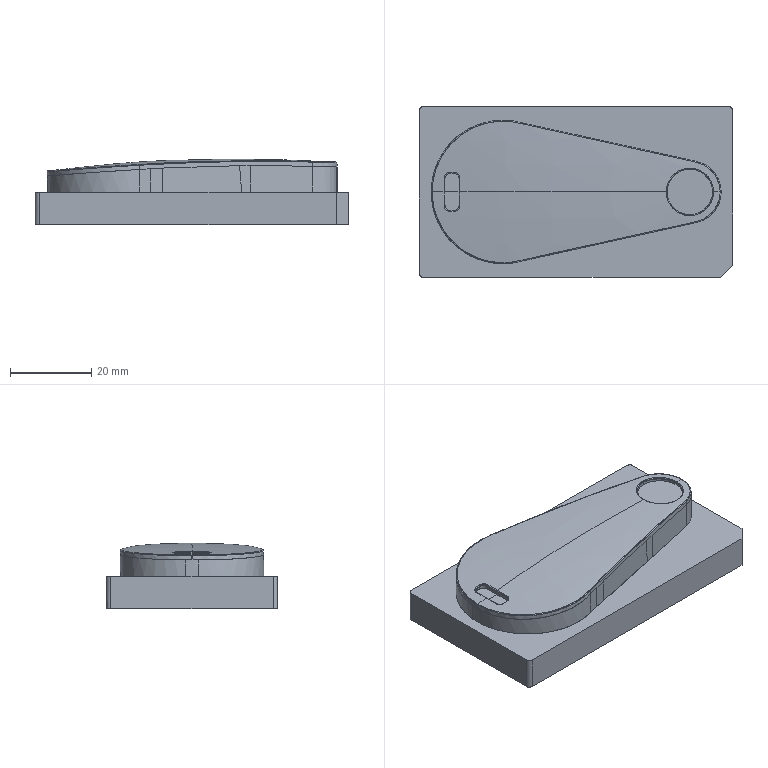NC program | PowerMill | posted with a generic post | part box 77 x 42 x 16.114 mm
Lines 1 to 941 of 134652:
%
O0001
N104 ( POWERMILL CB  : 2026004.0)
N105 ( POST VER      : 2026.0.0.5161)
N106 ( OPTION FILE   : FANUC)
N107 ( OUTPUT WORKPLANE : WORLD)
N108 (  )
N109 ( TOOL LIST )
N110 (---------------------------------------)
N111 ( NO. | ID        | DIA.| TIP RAD|LENGTH)
N112 (---------------------------------------)
N113 (    1|D10C_1_1   |10.0 |  0.0   |71.48 )
N114 (    2|D4C_2_1    | 4.0 |  0.0   |63.16 )
N115 (   28|D2C_1_1    | 2.0 |  0.0   |58.12 )
N116 (    3|D10_1_1    |10.0 |  0.0   | 71.2 )
N117 (    7|R2_2_1     | 4.0 |  2.0   | 60.4 )
N118 (   12|D2_1_1     | 2.0 |  0.0   |58.28 )
N119 (    6|R0.5_2_1   | 1.0 |  0.5   | 57.6 )
N120 (   13|TEXT_D4_1_1| 4.0 |  0.3   |63.36 )
N121 (---------------------------------------)
N122 (  )
N123 ( NUMBER OF TOOLPATHS: 15.0 )
N124 ( ESTIMATED PROGRAM DURATION: 0 HOURS 30 MIN 20 SEC)
N125 (  )
N126 G00 G21 G80 G40 G17
N127 G90
N128 G54
N129 G53 Z0.0
N130 (---------------)
N131 ( START TOOLPATH : 粗公开粗01-扫面平行-D10C )
N132 (---------------)
N133 ( TOOL NO.    :1 )
N134 ( TOOL TYPE   : ENDMILL)
N135 ( TOOL ID     : D10C_1_1)
N136 ( TOOL DIA    : 10.0 LENGTH 71.48)
N137 T1
N138 M6
N139 S8000 M03
N140 G00 G90 X0.0 Y0.0
N141 G43 Z10.6 H1
N142
N143 G05 P10000 R4
N144 X46.15 Y23.65
N145 Z1.4015
N146 G01 Z0.2015 F6000.0
N147 X41.15 F10000.0
N148 X-41.15
N149 Y17.7375
N150 X41.15
N151 Y11.825
N152 X-41.15
N153 Y5.9125
N154 X41.15
N155 Y0.0
N156 X-41.15
N157 Y-5.9125
N158 X41.15
N159 Y-11.825
N160 X-41.15
N161 Y-17.7375
N162 X41.15
N163 Y-23.65
N164 X-41.15
N165 X-46.15
N166 Z-0.197
N167 X-41.15
N168 X41.15
N169 Y-17.7375
N170 X-41.15
N171 Y-11.825
N172 X41.15
N173 Y-5.9125
N174 X-41.15
N175 Y0.0
N176 X41.15
N177 Y5.9125
N178 X-41.15
N179 Y11.825
N180 X41.15
N181 Y17.7375
N182 X-41.15
N183 Y23.65
N184 X41.15
N185 X46.15
N186 G00 Z10.6
N187 G05 P0
N188 (---------------)
N189 ( END TOOLPATH : 粗公开粗01-扫面平行-D10C )
N190 (---------------)
N191 ( START TOOLPATH : 粗公开粗01-外形偏置-D10C )
N192 (---------------)
N193 G00 X0.0415 Y-0.002 Z9.8037
N194 G05 P10000 R4
N195 X15.1122 Y-30.557
N196 Z0.5573
N197 G01 Z-0.6427 F6000.0
N198 Y-30.0295 F10000.0
N199 G03 X10.3647 Y-25.282 I-4.7475 J0.0
N200 G01 X-42.229
N201 G02 X-43.229 Y-24.282 I0.0 J1.0
N202 G01 Y-8.9867
N203 X-38.3097
N204 X-32.4189
N205 X-27.9189
N206 X-32.4189
N207 Y-12.472
N208 G03 X-30.5081 Y-14.47 I2.0 J0.0
N209 G01 X-22.4604 Y-14.8291
N210 G03 X-20.6866 Y-12.1962 I0.0829 J1.8581
N211 G01 X-21.7475 Y-9.8614
N212 G02 X-23.7344 Y-0.5015 I21.0967 J9.3693
N213 G01 X-23.7348 Y0.4347
N214 G02 X-22.8956 Y6.4023 I21.5767 J0.0088
N215 G01 X-22.6364 Y7.2526
N216 X-26.9406 Y8.5652
N217 X-22.6364 Y7.2526
N218 X-22.5842 Y7.4234
N219 G02 X-21.5821 Y10.0985 I28.7047 J-9.2284
N220 G01 X-20.6681 Y12.2256
N221 G03 X-22.4648 Y14.8251 I-1.7135 J0.7363
N222 G01 X-30.5081 Y14.466
N223 G03 X-32.4189 Y12.468 I0.0892 J-1.998
N224 G01 Y-8.9867
N225 X-38.3097
N226 Y19.8018
N227 G02 X-37.7528 Y20.3587 I0.5569 J0.0
N228 G01 X-2.203 Y20.3592
N229 G02 X-2.1341 Y19.97 I0.0 J-0.2007
N230 G01 X-4.361 Y19.1563
N231 G03 X-11.3917 Y14.9524 I7.4992 J-20.5229
N232 G01 X-12.0246 Y14.3889
N233 G03 X-16.1388 Y8.746 I10.9665 J-12.317
N234 G01 X-16.5756 Y7.7592
N235 G03 X-17.4466 Y5.3603 I17.0855 J-7.5614
N236 G01 X-17.5851 Y4.8788
N237 G03 X-18.21 Y0.4369 I15.427 J-4.4353
N238 G01 X-18.2096 Y-0.4993
N239 G03 X-16.6888 Y-7.6401 I17.5588 J0.0072
N240 G01 X-16.4205 Y-8.2422
N241 X-16.0824 Y-8.9571
N242 X-15.7125 Y-9.656
N243 X-15.4448 Y-10.1355
N244 G03 X-11.7963 Y-14.5782 I14.1498 J7.9007
N245 G01 X-10.8792 Y-15.3585
N246 G03 X-3.5709 Y-19.4506 I14.0407 J16.5038
N247 G01 X-1.9551 Y-19.9788
N248 G02 X-2.0163 Y-20.3632 I-0.0612 J-0.1873
N249 G01 X-37.7528 Y-20.3627
N250 G02 X-38.3097 Y-19.8058 I0.0 J0.5569
N251 G01 Y-8.9867
N252 X-43.229
N253 Y24.278
N254 G02 X-42.229 Y25.278 I1.0 J0.0
N255 G01 X42.312
N256 G02 X43.312 Y24.278 I0.0 J-1.0
N257 G01 Y-0.002
N258 X38.3927
N259 Y-19.8058
N260 G02 X37.8358 Y-20.3627 I-0.5569 J0.0
N261 G01 X19.3428 Y-20.3632
N262 G02 X19.3059 Y-20.0003 I0.0 J0.1833
N263 G01 X25.8243 Y-18.6576
N264 G03 X35.9604 Y-11.8793 I-3.2646 J15.8493
N265 G01 X36.1512 Y-11.5973
N266 X36.2852 Y-11.3934
N267 X36.4135 Y-11.186
N268 X36.5859 Y-10.8987
N269 X36.7924 Y-10.5378
N270 G03 X38.0247 Y-5.4294 I-8.4899 J4.7508
N271 G01 X38.0231 Y-5.3865
N272 G03 X37.0167 Y-1.4345 I-9.6578 J-0.3552
N273 G01 X36.9442 Y-1.2889
N274 X36.7974 Y-1.0108
N275 X36.6375 Y-0.74
N276 X36.5527 Y-0.6039
N277 G02 X36.5528 Y0.6042 I0.9695 J0.604
N278 G01 X36.6374 Y0.74
N279 X36.877 Y1.1579
N280 X37.0853 Y1.5923
N281 X37.228 Y1.92
N282 G03 X37.2314 Y9.6259 I-8.8607 J3.8569
N283 G01 X37.0921 Y9.9456
N284 G03 X35.1033 Y12.9253 I-9.3798 J-4.1071
N285 G01 X33.7038 Y14.3849
N286 X33.546 Y14.5438
N287 G03 X26.2035 Y18.5373 I-10.3837 J-10.3447
N288 G01 X19.3237 Y19.9965
N289 G02 X19.3617 Y20.3592 I0.038 J0.1794
N290 G01 X37.8358 Y20.3587
N291 G02 X38.3927 Y19.8018 I0.0 J-0.5569
N292 G01 Y-0.002
N293 X43.312
N294 Y-24.282
N295 G02 X42.312 Y-25.282 I-1.0 J0.0
N296 G01 X10.3647
N297 X10.096 Y-16.8337
N298 X9.3226 Y-16.8583
N299 X7.0023 Y-16.7279
N300 X6.2289 Y-16.6328
N301 X3.9086 Y-16.2963
N302 X1.5884 Y-15.9314
N303 X0.8149 Y-15.7235
N304 X0.0415 Y-15.472
N305 X-1.0167 Y-15.0838
N306 X-1.5054 Y-14.9304
N307 X-3.8256 Y-14.0783
N308 X-4.7965 Y-13.537
N309 X-6.09 Y-12.7635
N310 X-8.4662 Y-10.8994
N311 X-9.2396 Y-10.254
N312 X-10.013 Y-9.3444
N313 X-11.3207 Y-7.3496
N314 X-11.7729 Y-6.5761
N315 X-12.3692 Y-5.0293
N316 X-12.8353 Y-3.4824
N317 X-12.9849 Y-2.709
N318 X-13.1446 Y-1.1621
N319 X-13.261 Y-0.3887
N320 X-13.2613 Y0.3847
N321 X-13.1068 Y1.4875
N322 X-12.7819 Y3.4784
N323 X-12.6318 Y4.2518
N324 X-12.3829 Y5.0253
N325 X-12.0531 Y5.7987
N326 X-11.2708 Y7.3456
N327 X-10.7865 Y8.1825
N328 X-10.013 Y9.3424
N329 X-9.2396 Y10.2581
N330 X-8.4662 Y10.9107
N331 X-6.1459 Y12.7679
N332 X-5.3725 Y13.2565
N333 X-4.5991 Y13.704
N334 X-3.8256 Y14.0474
N335 X0.0415 Y15.5415
N336 X0.8149 Y15.7355
N337 X4.6821 Y16.4562
N338 X7.7758 Y16.7747
N339 X9.3226 Y16.8711
N340 X10.096 Y16.8388
N341 X10.8695 Y16.7141
N342 X13.1898 Y16.2845
N343 X20.1506 Y14.7825
N344 X24.7911 Y13.7125
N345 X27.1114 Y13.0685
N346 X27.8849 Y12.7169
N347 X28.9862 Y11.9861
N348 X30.2051 Y10.9294
N349 X31.4204 Y9.6658
N350 X32.0706 Y8.8924
N351 X32.5169 Y8.119
N352 X32.8414 Y7.3456
N353 X33.0385 Y6.5721
N354 X33.1043 Y5.7987
N355 X33.0532 Y5.0253
N356 X32.854 Y4.2518
N357 X32.5404 Y3.4784
N358 X32.0786 Y2.705
N359 X31.3653 Y1.9316
N360 X30.9786 Y1.661
N361 X30.1787 Y1.1581
N362 X29.4317 Y0.8897
N363 X28.6583 Y0.6895
N364 X28.0947 Y0.573
N365 X28.0184 Y0.5508
N366 X27.9466 Y0.5168
N367 X27.8039 Y0.4348
N368 X27.7235 Y0.3772
N369 X27.6559 Y0.3049
N370 X27.6546 Y0.3032
N371 G03 X27.8164 Y-0.4416 I0.3972 J-0.3037
N372 G01 X27.9881 Y-0.5332
N373 X28.0482 Y-0.5603
N374 X28.1114 Y-0.5793
N375 X29.4317 Y-0.8831
N376 X30.2051 Y-1.1867
N377 X30.9786 Y-1.6615
N378 X31.37 Y-1.9356
N379 X32.0818 Y-2.709
N380 X32.5426 Y-3.4824
N381 X32.8554 Y-4.2558
N382 X33.0533 Y-5.0293
N383 X33.1042 Y-5.8027
N384 X33.0378 Y-6.5761
N385 X32.8256 Y-7.3496
N386 X32.5042 Y-8.123
N387 X32.0402 Y-8.8964
N388 X31.41 Y-9.6698
N389 X30.6871 Y-10.4433
N390 X30.2051 Y-10.917
N391 X29.4317 Y-11.6072
N392 X28.6583 Y-12.2299
N393 X27.83 Y-12.7635
N394 X27.1114 Y-13.0685
N395 X26.338 Y-13.2989
N396 X24.7911 Y-13.7128
N397 X20.1506 Y-14.7825
N398 X13.1898 Y-16.2844
N399 X11.341 Y-16.6307
N400 X10.096 Y-16.8337
N401 X10.3647 Y-25.282
N402 G00 Z3.2117
N403 G01 X15.1122 Y-30.557
N404 G00 Z0.1617
N405 G01 Z-1.0383 F6000.0
N406 Y-30.0295 F10000.0
N407 G03 X10.3647 Y-25.282 I-4.7475 J0.0
N408 G01 X-30.4481
N409 X-30.0672 Y-20.5382
N410 X-29.6209 Y-14.9804
N411 G03 X-27.5814 Y-12.3027 I0.1601 J1.9936
N412 G01 X-28.0999 Y-10.8534
N413 G02 X-28.0952 Y10.9505 I30.7936 J10.8953
N414 G01 X-27.6041 Y12.3366
N415 G03 X-30.1715 Y14.8846 I-1.8852 J0.6679
N416 G01 X-31.2015 Y14.5108
N417 G03 X-32.5193 Y12.6308 I0.6822 J-1.88
N418 G01 Y-12.6347
N419 G03 X-31.1506 Y-14.5324 I2.0 J0.0
N420 G01 X-30.0921 Y-14.8845
N421 X-29.8594 Y-14.9467
N422 X-29.6209 Y-14.9804
N423 X-30.0672 Y-20.5382
N424 X-36.4389 Y-20.4705
N425 G02 X-38.4176 Y-18.4706 I0.0213 J1.9999
N426 G01 Y18.4666
N427 G02 X-36.4389 Y20.4665 I2.0 J0.0
N428 G01 X-17.4527 Y20.6686
N429 G02 X-16.606 Y18.6466 I0.0126 J-1.183
N430 G01 X-17.0632 Y18.1921
N431 G03 X-24.3705 Y1.1083 I17.475 J-17.5793
N432 G01 X-24.3798 Y0.6397
N433 G03 X-22.711 Y-9.5229 I28.3295 J-0.5663
N434 G01 X-22.5542 Y-9.9586
N435 X-22.3535 Y-10.4413
N436 G03 X-17.4562 Y-17.7416 I21.2986 J8.9951
N437 G01 X-16.5667 Y-18.6369
N438 G02 X-17.4265 Y-20.6726 I-0.8471 J-0.8416
N439 G01 X-30.0672 Y-20.5382
N440 X-30.4481 Y-25.282
N441 X-42.229
N442 G02 X-43.229 Y-24.282 I0.0 J1.0
N443 G01 Y24.278
N444 G02 X-42.229 Y25.278 I1.0 J0.0
N445 G01 X23.2539
N446 X23.1838 Y20.6695
N447 X36.531 Y20.4664
N448 G02 X38.4897 Y18.6752 I-0.0304 J-1.9998
N449 G01 X38.6939 Y16.7285
N450 G02 X36.5553 Y15.2042 I-1.5004 J-0.1574
N451 G01 X35.0306 Y15.9161
N452 G03 X23.8289 Y18.8401 I-13.5676 J-29.0589
N453 G01 X23.1047 Y18.8937
N454 G02 X23.1838 Y20.6695 I0.0656 J0.8867
N455 G01 X23.2539 Y25.278
N456 X42.312
N457 G02 X43.312 Y24.278 I0.0 J-1.0
N458 G01 Y0.8328
N459 X40.7182 Y0.6747
N460 X40.7359 Y0.3847
N461 X40.7358 Y-0.3887
N462 X40.6884 Y-1.1621
N463 X40.5966 Y-1.9356
N464 X40.4561 Y-2.709
N465 X40.267 Y-3.4824
N466 X40.024 Y-4.2558
N467 X39.7231 Y-5.0293
N468 X39.4863 Y-5.5542
N469 X38.7128 Y-6.9415
N470 X37.9394 Y-8.0197
N471 X37.1697 Y-8.8964
N472 X36.3925 Y-9.6404
N473 X35.6191 Y-10.2695
N474 X34.8457 Y-10.8012
N475 X34.1495 Y-11.2167
N476 X33.3841 Y-11.5997
N477 X35.0209 Y-15.888
N478 X35.3181 Y-15.7746
N479 X36.5715 Y-15.2009
N480 G02 X38.694 Y-16.72 I0.6291 J-1.3633
N481 G01 X38.4898 Y-18.678
N482 G02 X36.531 Y-20.4704 I-1.9892 J0.2074
N483 G01 X23.1804 Y-20.6735
N484 G02 X22.9728 Y-18.9175 I-0.0136 J0.8887
N485 G01 X32.941 Y-16.6819
N486 X35.0209 Y-15.888
N487 X33.3841 Y-11.5997
N488 X33.2988 Y-11.6423
N489 X32.5254 Y-11.9652
N490 X31.752 Y-12.235
N491 X30.9786 Y-12.4436
N492 X2.3618 Y-18.762
N493 X0.0415 Y-19.25
N494 X-1.5054 Y-19.544
N495 X-2.6219 Y-19.7244
N496 X-3.8256 Y-19.8165
N497 X-4.5991 Y-19.7629
N498 X-4.8522 Y-19.7244
N499 X-5.3725 Y-19.589
N500 X-7.6928 Y-18.7837
N501 X-8.4662 Y-18.4131
N502 X-10.4024 Y-17.4041
N503 X-10.7865 Y-17.1736
N504 X-12.3333 Y-16.1446
N505 X-12.7128 Y-15.8572
N506 X-13.1068 Y-15.5181
N507 X-14.3773 Y-14.3104
N508 X-14.6536 Y-13.9962
N509 X-16.2005 Y-12.0628
N510 X-16.807 Y-11.2167
N511 X-17.2476 Y-10.4433
N512 X-17.6483 Y-9.6698
N513 X-18.3347 Y-8.123
N514 X-19.0377 Y-5.8027
N515 X-19.2168 Y-5.0293
N516 X-19.6216 Y-2.709
N517 X-19.7892 Y-0.3887
N518 X-19.7895 Y0.3847
N519 X-19.5257 Y3.4784
N520 X-19.4179 Y4.2518
N521 X-19.239 Y5.0253
N522 X-18.3485 Y8.119
N523 X-18.0172 Y8.8924
N524 X-17.2664 Y10.4393
N525 X-16.8106 Y11.2127
N526 X-15.6959 Y12.7595
N527 X-14.6536 Y14.0091
N528 X-13.8802 Y14.8285
N529 X-12.7132 Y15.8532
N530 X-11.5599 Y16.6885
N531 X-10.7865 Y17.1653
N532 X-8.4662 Y18.4161
N533 X-7.6928 Y18.781
N534 X-5.3725 Y19.5813
N535 X-4.8744 Y19.7204
N536 X-4.5991 Y19.7641
N537 X-3.8256 Y19.8171
N538 X-2.5558 Y19.7204
N539 X0.0415 Y19.2508
N540 X2.3618 Y18.7622
N541 X30.9786 Y12.4427
N542 X31.752 Y12.2338
N543 X32.5254 Y11.9643
N544 X33.2988 Y11.6448
N545 X34.0723 Y11.2583
N546 X34.8457 Y10.7997
N547 X35.3878 Y10.4393
N548 X36.3925 Y9.6409
N549 X37.166 Y8.9002
N550 X37.8572 Y8.119
N551 X38.7128 Y6.9413
N552 X39.3664 Y5.7987
N553 X39.7262 Y5.0253
N554 X40.0224 Y4.2518
N555 X40.2597 Y3.5067
N556 X40.4569 Y2.705
N557 X40.5969 Y1.9316
N558 X40.6888 Y1.1581
N559 X40.7182 Y0.6747
N560 X43.312 Y0.8328
N561 Y-24.282
N562 G02 X42.312 Y-25.282 I-1.0 J0.0
N563 G01 X10.3647
N564 G00 Z2.8161
N565 G01 X15.1122 Y-30.557
N566 G00 Z-0.2339
N567 G01 Z-1.4339 F6000.0
N568 Y-30.0295 F10000.0
N569 G03 X10.3647 Y-25.282 I-4.7475 J0.0
N570 G01 X-42.229
N571 G02 X-43.229 Y-24.282 I0.0 J1.0
N572 G01 Y-11.6956
N573 X-38.4176
N574 X-33.9176
N575 X-38.4176
N576 Y18.4666
N577 G02 X-36.4524 Y20.4663 I2.0 J0.0
N578 G01 X-24.8529 Y20.6681
N579 G02 X-23.7 Y18.5172 I0.0239 J-1.3716
N580 G01 X-24.0873 Y17.956
N581 G03 X-27.7221 Y10.5034 I22.7817 J-15.7237
N582 G01 X-32.0165 Y11.8481
N583 X-27.7221 Y10.5034
N584 G03 X-28.7894 Y5.5313 I26.4164 J-8.2712
N585 G01 X-28.9335 Y4.3307
N586 G03 X-27.0613 Y-12.1403 I35.6942 J-4.2847
N587 G01 X-26.9601 Y-12.4213
N588 G03 X-24.4575 Y-17.3996 I21.8992 J7.8905
N589 G01 X-23.7024 Y-18.5378
N590 G02 X-24.8717 Y-20.6721 I-1.1454 J-0.7599
N591 G01 X-36.4525 Y-20.4703
N592 G02 X-38.4176 Y-18.4706 I0.0349 J1.9997
N593 G01 Y-11.6956
N594 X-43.229
N595 Y24.278
N596 G02 X-42.229 Y25.278 I1.0 J0.0
N597 G01 X23.3241
N598 X23.2536 Y20.6695
N599 X36.5312 Y20.4664
N600 G02 X38.4895 Y18.6768 I-0.0306 J-1.9998
N601 G01 X38.6938 Y16.7446
N602 G02 X36.5442 Y15.2346 I-1.4942 J-0.1579
N603 G01 X34.9168 Y16.0234
N604 G03 X23.8813 Y18.858 I-12.5129 J-25.8153
N605 G01 X23.1943 Y18.8935
N606 G02 X23.2536 Y20.6695 I0.0457 J0.8874
N607 G01 X23.3241 Y25.278
N608 X42.312
N609 G02 X43.312 Y24.278 I0.0 J-1.0
N610 G01 Y0.8214
N611 X40.7633 Y0.6747
N612 X40.78 Y0.3847
N613 X40.7828 Y-0.3887
N614 X40.7377 Y-1.1621
N615 X40.6416 Y-1.9356
N616 X40.4956 Y-2.709
N617 X40.3048 Y-3.4824
N618 X40.0636 Y-4.2558
N619 X39.76 Y-5.0293
N620 X39.4863 Y-5.6228
N621 X38.9706 Y-6.5761
N622 X38.7128 Y-6.9935
N623 X37.9394 Y-8.0609
N624 X37.2013 Y-8.8964
N625 X36.3925 Y-9.6652
N626 X35.6191 Y-10.2892
N627 X34.8457 Y-10.8205
N628 X34.0723 Y-11.2707
N629 X33.2988 Y-11.6539
N630 X32.5254 Y-11.98
N631 X31.752 Y-12.2506
N632 X30.9786 Y-12.4599
N633 X-6.9193 Y-20.8129
N634 X-9.2297 Y-21.2712
N635 X-10.013 Y-21.3992
N636 X-10.7865 Y-21.4871
N637 X-11.5599 Y-21.5111
N638 X-12.3333 Y-21.4423
N639 X-13.1068 Y-21.2636
N640 X-13.8802 Y-20.9409
N641 X-14.6536 Y-20.5276
N642 X-15.427 Y-20.0047
N643 X-16.8355 Y-18.9509
N644 X-17.7473 Y-18.2498
N645 X-18.5207 Y-17.5178
N646 X-19.9516 Y-15.8572
N647 X-20.4829 Y-15.0838
N648 X-21.3738 Y-13.537
N649 X-21.7882 Y-12.7635
N650 X-22.7935 Y-10.4433
N651 X-23.0558 Y-9.6698
N652 X-23.1613 Y-9.2762
N653 X-23.5442 Y-8.123
N654 X-23.7474 Y-7.3496
N655 X-23.8731 Y-6.5761
N656 X-23.8744 Y-6.569
N657 X-24.1709 Y-5.0293
N658 X-24.4369 Y-2.709
N659 X-24.5518 Y-0.3887
N660 X-24.5511 Y0.3847
N661 X-24.3719 Y3.4784
N662 X-24.2725 Y4.2518
N663 X-23.9347 Y6.2496
N664 X-23.8607 Y6.5721
N665 X-23.7435 Y7.3456
N666 X-23.5425 Y8.119
N667 X-23.1613 Y9.4126
N668 X-22.7954 Y10.4393
N669 X-22.3879 Y11.468
N670 X-21.7958 Y12.7595
N671 X-21.391 Y13.533
N672 X-20.4829 Y15.0798
N673 X-19.9456 Y15.8532
N674 X-18.5945 Y17.4001
N675 X-17.7473 Y18.2185
N676 X-16.9739 Y18.8924
N677 X-15.8964 Y19.7204
N678 X-15.427 Y20.027
N679 X-13.8802 Y20.9344
N680 X-13.1068 Y21.2567
N681 X-12.3333 Y21.4456
N682 X-11.5599 Y21.5105
N683 X-10.7865 Y21.4823
N684 X-10.013 Y21.3987
N685 X-9.2058 Y21.2672
N686 X-6.9193 Y20.8129
N687 X0.0415 Y19.2877
N688 X30.9786 Y12.4601
N689 X31.752 Y12.2506
N690 X32.5064 Y11.9861
N691 X33.2988 Y11.6536
N692 X34.0723 Y11.2709
N693 X34.8457 Y10.8207
N694 X35.4057 Y10.4393
N695 X36.3918 Y9.6658
N696 X37.2052 Y8.8924
N697 X37.8912 Y8.119
N698 X38.7128 Y6.9933
N699 X39.3968 Y5.7987
N700 X39.7607 Y5.0253
N701 X40.065 Y4.2518
N702 X40.3065 Y3.4784
N703 X40.4953 Y2.705
N704 X40.6423 Y1.9316
N705 X40.7355 Y1.1581
N706 X40.7633 Y0.6747
N707 X43.312 Y0.8214
N708 Y-17.2259
N709 X38.6938 Y-16.7399
N710 X38.4896 Y-18.68
N711 G02 X36.5313 Y-20.4704 I-1.989 J0.2094
N712 G01 X23.284 Y-20.6735
N713 G02 X23.079 Y-18.9201 I-0.0136 J0.8871
N714 G01 X31.9522 Y-16.9599
N715 X32.3633 Y-16.8546
N716 G03 X35.2885 Y-15.8067 I-4.3383 J16.7172
N717 G01 X36.5628 Y-15.216
N718 G02 X38.6938 Y-16.7399 I0.6334 J-1.3662
N719 G01 X43.312 Y-17.2259
N720 Y-24.282
N721 G02 X42.312 Y-25.282 I-1.0 J0.0
N722 G01 X10.3647
N723 G00 Z2.4204
N724 G01 X15.1122 Y-30.557
N725 G00 Z-0.6296
N726 G01 Z-1.8296 F6000.0
N727 Y-30.0295 F10000.0
N728 G03 X10.3647 Y-25.282 I-4.7475 J0.0
N729 G01 X-42.229
N730 G02 X-43.229 Y-24.282 I0.0 J1.0
N731 G01 Y24.278
N732 G02 X-42.229 Y25.278 I1.0 J0.0
N733 G01 X23.4146
N734 X23.3436 Y20.6695
N735 X36.5314 Y20.4664
N736 G02 X38.4894 Y18.6785 I-0.0308 J-1.9998
N737 G01 X38.6936 Y16.7615
N738 G02 X36.5594 Y15.2357 I-1.4984 J-0.1596
N739 G01 X35.066 Y15.9306
N740 G03 X23.9862 Y18.838 I-13.5769 J-29.1746
N741 G01 X23.261 Y18.8945
N742 G02 X23.3436 Y20.6695 I0.0689 J0.8862
N743 G01 X23.4146 Y25.278
N744 X42.312
N745 G02 X43.312 Y24.278 I0.0 J-1.0
N746 G01 Y0.827
N747 X40.7784 Y0.6747
N748 X40.7958 Y0.3847
N749 X40.7936 Y-0.3887
N750 X40.7515 Y-1.1621
N751 X40.6555 Y-1.9356
N752 X40.5108 Y-2.709
N753 X40.3193 Y-3.4824
N754 X40.0782 Y-4.2558
N755 X39.775 Y-5.0293
N756 X39.4863 Y-5.6524
N757 X38.9856 Y-6.5761
N758 X38.7128 Y-7.0195
N759 X37.9394 Y-8.0827
N760 X37.2207 Y-8.8964
N761 X36.4087 Y-9.6698
N762 X35.6191 Y-10.3064
N763 X34.8457 Y-10.837
N764 X34.0723 Y-11.2865
N765 X33.2988 Y-11.6693
N766 X32.5254 Y-11.9943
N767 X31.7572 Y-12.2632
N768 X33.1106 Y-16.657
N769 G03 X35.2872 Y-15.8223 I-5.0931 J16.5352
N770 G01 X36.5623 Y-15.2319
N771 G02 X38.6937 Y-16.7582 I0.6331 J-1.3672
N772 G01 X38.4894 Y-18.6818
N773 G02 X36.5314 Y-20.4704 I-1.9888 J0.2112
N774 G01 X23.3413 Y-20.6735
N775 G02 X23.1365 Y-18.9202 I-0.0136 J0.887
N776 G01 X31.9513 Y-16.9745
N777 X32.363 Y-16.869
N778 X32.738 Y-16.7672
N779 X33.1106 Y-16.657
N780 X31.7572 Y-12.2632
N781 X31.752 Y-12.265
N782 X30.9786 Y-12.4743
N783 X30.2051 Y-12.6511
N784 X-11.5599 Y-21.8421
N785 X-11.5687 Y-21.8444
N786 X-12.3434 Y-22.0447
N787 X-13.1068 Y-22.2252
N788 X-13.8802 Y-22.3746
N789 X-15.427 Y-22.5766
N790 X-16.9739 Y-22.6242
N791 X-17.7473 Y-22.5698
N792 X-18.5207 Y-22.44
N793 X-19.2942 Y-22.2113
N794 X-19.6836 Y-22.0447
N795 X-20.0676 Y-21.836
N796 X-20.841 Y-21.2908
N797 X-21.6144 Y-20.59
N798 X-22.3879 Y-19.8338
N799 X-23.1756 Y-18.9509
N800 X-24.3226 Y-17.4041
N801 X-24.8131 Y-16.6307
N802 X-24.9059 Y-16.4451
N803 X-29.0506 Y-18.4187
N804 G02 X-30.5267 Y-20.6711 I-1.4228 J-0.6774
N805 G01 X-36.4853 Y-20.4695
N806 G02 X-38.4176 Y-18.4706 I0.0677 J1.9989
N807 G01 Y18.4666
N808 G02 X-36.4287 Y20.4666 I2.0 J0.0
N809 G01 X-30.189 Y20.5011
N810 G02 X-29.0624 Y18.8107 I0.0068 J-1.2161
N811 G01 X-30.4931 Y15.4335
N812 G03 X-33.2626 Y0.5768 I32.4046 J-13.7272
N813 G01 X-33.2106 Y-1.044
N814 X-33.079 Y-3.7544
N815 G03 X-29.7256 Y-17.0012 I34.9556 J1.8011
N816 G01 X-29.0506 Y-18.4187
N817 X-24.9059 Y-16.4451
N818 X-25.4816 Y-15.2938
N819 X-25.9563 Y-14.3104
N820 X-26.5667 Y-12.7635
N821 X-26.8389 Y-11.9901
N822 X-27.4816 Y-9.6698
N823 X-27.9788 Y-7.3496
N824 X-28.3112 Y-5.0293
N825 X-28.5162 Y-2.709
N826 X-28.5966 Y-0.3887
N827 X-28.5901 Y0.3847
N828 X-28.4636 Y3.4784
N829 X-28.1905 Y5.7987
N830 X-27.9648 Y7.3456
N831 X-27.483 Y9.6658
N832 X-26.84 Y11.9861
N833 X-26.5684 Y12.7595
N834 X-25.9483 Y14.3064
N835 X-25.2183 Y15.8532
N836 X-24.3124 Y17.4001
N837 X-23.2168 Y18.9469
N838 X-22.5194 Y19.7204
N839 X-20.841 Y21.2762
N840 X-20.0676 Y21.8439
N841 X-19.6956 Y22.0407
N842 X-19.2942 Y22.2087
N843 X-18.5207 Y22.4408
N844 X-17.7473 Y22.5659
N845 X-16.9739 Y22.6234
N846 X-16.2005 Y22.6159
N847 X-15.427 Y22.5767
N848 X-13.8802 Y22.3745
N849 X-13.1068 Y22.2253
N850 X-11.5599 Y21.8421
N851 X6.2289 Y17.943
N852 X30.9786 Y12.4742
N853 X31.752 Y12.265
N854 X32.5254 Y11.9939
N855 X33.2988 Y11.6688
N856 X34.0723 Y11.287
N857 X34.8457 Y10.8371
N858 X35.4302 Y10.4393
N859 X36.3925 Y9.6833
N860 X37.166 Y8.9521
N861 X37.9394 Y8.0827
N862 X38.4912 Y7.3456
N863 X38.9872 Y6.5721
N864 X39.4122 Y5.7987
N865 X39.7756 Y5.0253
N866 X40.0796 Y4.2518
N867 X40.3221 Y3.4784
N868 X40.5112 Y2.705
N869 X40.6564 Y1.9316
N870 X40.7494 Y1.1581
N871 X40.7784 Y0.6747
N872 X43.312 Y0.827
N873 Y-24.282
N874 G02 X42.312 Y-25.282 I-1.0 J0.0
N875 G01 X10.3647
N876 G00 Z2.0247
N877 G01 X15.1122 Y-30.557
N878 G00 Z-1.0252
N879 G01 Z-2.2253 F6000.0
N880 Y-30.0295 F10000.0
N881 G03 X10.3647 Y-25.282 I-4.7475 J0.0
N882 G01 X-42.229
N883 G02 X-43.229 Y-24.282 I0.0 J1.0
N884 G01 Y-0.002
N885 X-38.1046
N886 Y19.2869
N887 G02 X-37.2379 Y20.1536 I0.8667 J0.0
N888 G01 X-34.1272 Y20.1539
N889 G02 X-33.6391 Y19.392 I0.0001 J-0.5372
N890 G01 X-33.8097 Y19.0215
N891 G03 X-35.6143 Y14.0445 I28.7694 J-13.2468
N892 G01 X-35.749 Y13.5463
N893 G03 X-37.4205 Y-3.3019 I49.6691 J-13.4347
N894 G01 X-37.3852 Y-3.8335
N895 G03 X-35.0608 Y-15.8669 I49.2716 J3.2761
N896 G01 X-35.0111 Y-16.0194
N897 G03 X-33.8739 Y-18.8832 I23.3493 J7.6142
N898 G01 X-33.6281 Y-19.4043
N899 G02 X-34.1059 Y-20.1579 I-0.4777 J-0.2254
N900 G01 X-37.2379 Y-20.1576
N901 G02 X-38.1046 Y-19.2909 I0.0 J0.8667
N902 G01 Y-0.002
N903 X-43.229
N904 Y24.278
N905 G02 X-42.229 Y25.278 I1.0 J0.0
N906 G01 X29.9707
N907 X29.9704 Y20.154
N908 X37.3209 Y20.1536
N909 G02 X38.1876 Y19.2869 I0.0 J-0.8667
N910 G01 X38.1879 Y15.6751
N911 G02 X37.456 Y15.2603 I-0.4834 J-0.0001
N912 G01 X37.1928 Y15.418
N913 G03 X31.904 Y17.522 I-9.118 J-15.22
N914 G01 X22.558 Y19.5878
N915 G02 X22.6199 Y20.1544 I0.0619 J0.2799
N916 G01 X29.9704 Y20.154
N917 X29.9707 Y25.278
N918 X42.312
N919 G02 X43.312 Y24.278 I0.0 J-1.0
N920 G01 Y0.3861
N921 X40.8095 Y0.3847
N922 X40.8099 Y-0.3887
N923 X40.7635 Y-1.1621
N924 X40.668 Y-1.9356
N925 X40.5237 Y-2.709
N926 X40.334 Y-3.4824
N927 X40.0903 Y-4.2558
N928 X39.7892 Y-5.0293
N929 X39.4282 Y-5.8027
N930 X39.0004 Y-6.5761
N931 X38.7128 Y-7.0391
N932 X37.9394 Y-8.0983
N933 X37.2337 Y-8.8964
N934 X36.4226 Y-9.6698
N935 X35.6191 Y-10.3166
N936 X34.8457 Y-10.8461
N937 X34.2235 Y-11.2167
N938 X33.2988 Y-11.681
N939 X32.5678 Y-11.9901
N940 X31.752 Y-12.2709
N941 X30.9786 Y-12.4795
N942 X30.3346 Y-12.6215
N943 X30.2051 Y-12.6511
N944 X27.3119 Y-13.2878
N945 X-11.5599 Y-21.8563
N946 X-12.3157 Y-22.0447
N947 X-13.1068 Y-22.2393
N948 X-14.6536 Y-22.5156
N949 X-16.2005 Y-22.684
N950 X-17.7473 Y-22.7514
N951 X-19.2942 Y-22.7097
N952 X-20.841 Y-22.5582
N953 X-22.3879 Y-22.296
N954 X-23.4312 Y-22.0447
N955 X-24.7081 Y-21.6218
N956 X-25.5174 Y-21.2712
N957 X-26.255 Y-20.8546
N958 X-26.7519 Y-20.4978
N959 X-27.0284 Y-20.2513
N960 X-27.5221 Y-19.7244
N961 X-27.8019 Y-19.3446
N962 X-28.4972 Y-18.1775
N963 X-29.2755 Y-16.6307
N964 X-29.6164 Y-15.8572
N965 X-30.1825 Y-14.3104
N966 X-30.8737 Y-11.9901
N967 X-31.0724 Y-11.2167
N968 X-31.5811 Y-8.8964
N969 X-31.9559 Y-6.5761
N970 X-32.1457 Y-5.0293
N971 X-32.2765 Y-3.4824
N972 X-32.4058 Y-0.3887
N973 X-32.3693 Y1.9316
N974 X-32.2186 Y4.2518
N975 X-31.9521 Y6.5721
N976 X-31.5814 Y8.8924
N977 X-31.0784 Y11.2127
N978 X-30.4277 Y13.533
N979 X-30.1756 Y14.3064
N980 X-29.6165 Y15.8532
N981 X-28.9128 Y17.4001
N982 X-28.5047 Y18.1735
N983 X-28.0406 Y18.9469
N984 X-27.5156 Y19.7204
N985 X-27.0284 Y20.2452
N986 X-26.7497 Y20.4938
N987 X-26.255 Y20.8514
N988 X-25.4816 Y21.2891
N989 X-24.7081 Y21.6231
N990 X-23.1613 Y22.1157
N991 X-21.6144 Y22.4463
N992 X-20.841 Y22.5584
N993 X-19.2942 Y22.7103
N994 X-17.7473 Y22.7483
N995 X-16.9739 Y22.7286
N996 X-16.2005 Y22.6787
N997 X-14.6536 Y22.5133
N998 X-13.1068 Y22.2394
N999 X-11.5599 Y21.8563
N1000 X-11.5532 Y21.8548
N1001 X-3.0522 Y19.9944
N1002 X30.2051 Y12.6556
N1003 X30.5863 Y12.5608
N1004 X30.9785 Y12.4741
N1005 X31.48 Y12.3385
N1006 X31.752 Y12.2708
N1007 X32.5254 Y12.0058
N1008 X33.2988 Y11.6805
N1009 X34.0723 Y11.2979
N1010 X34.8457 Y10.8464
N1011 X35.4448 Y10.4393
N1012 X36.4274 Y9.6658
N1013 X37.166 Y8.9667
N1014 X37.9222 Y8.119
N1015 X38.5043 Y7.3456
N1016 X39.0027 Y6.5721
N1017 X39.4304 Y5.7987
N1018 X39.7914 Y5.0253
N1019 X40.0916 Y4.2518
N1020 X40.3352 Y3.4784
N1021 X40.5246 Y2.705
N1022 X40.6685 Y1.9316
N1023 X40.7637 Y1.1581
N1024 X40.8095 Y0.3847
N1025 X43.312 Y0.3861
N1026 Y-24.282
N1027 G02 X42.312 Y-25.282 I-1.0 J0.0
N1028 G01 X29.9478
N1029 X29.9476 Y-20.158
N1030 X22.5742 Y-20.1584
N1031 G02 X22.5125 Y-19.5923 I0.0 J0.2864
N1032 G01 X31.8895 Y-17.525
N1033 G03 X35.6172 Y-16.249 I-3.7683 J17.0923
N1034 G01 X35.7848 Y-16.1696
N1035 X36.4144 Y-15.854
N1036 X37.0294 Y-15.5108
N1037 X37.4608 Y-15.2574
N1038 G02 X38.1879 Y-15.6737 I0.2445 J-0.4162